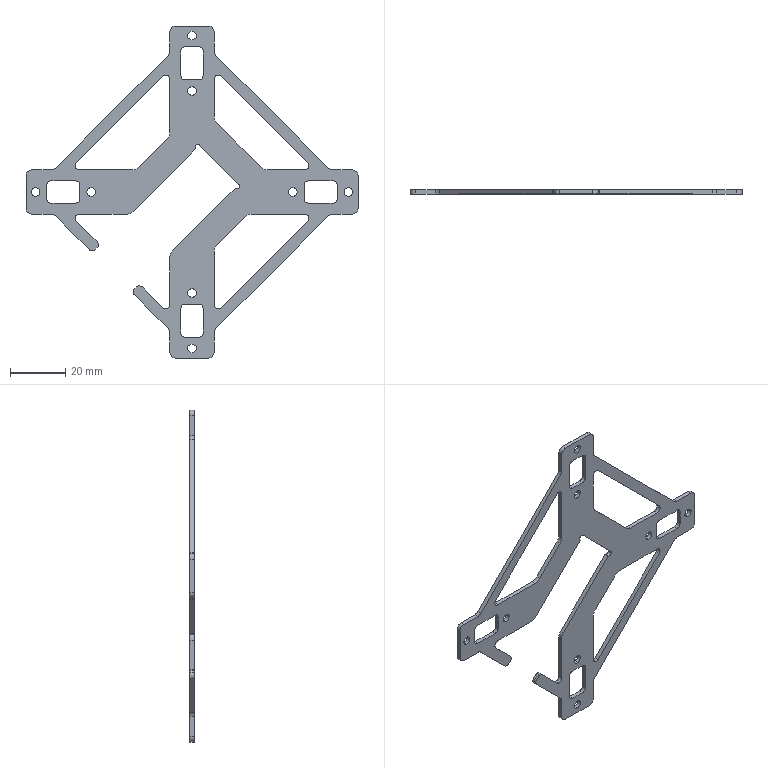Part | SolidWorks | features Fillet 3, Extrusion 1, ICE 1 | 1 solid | 130 faces | box 120 x 1.5 x 120 mm | volume 5507 mm3 | cylinder 74 | plane 56 | commonest cylinder face diameters 3 x31 3.1 x16 4 x16 6 x8 2 x3